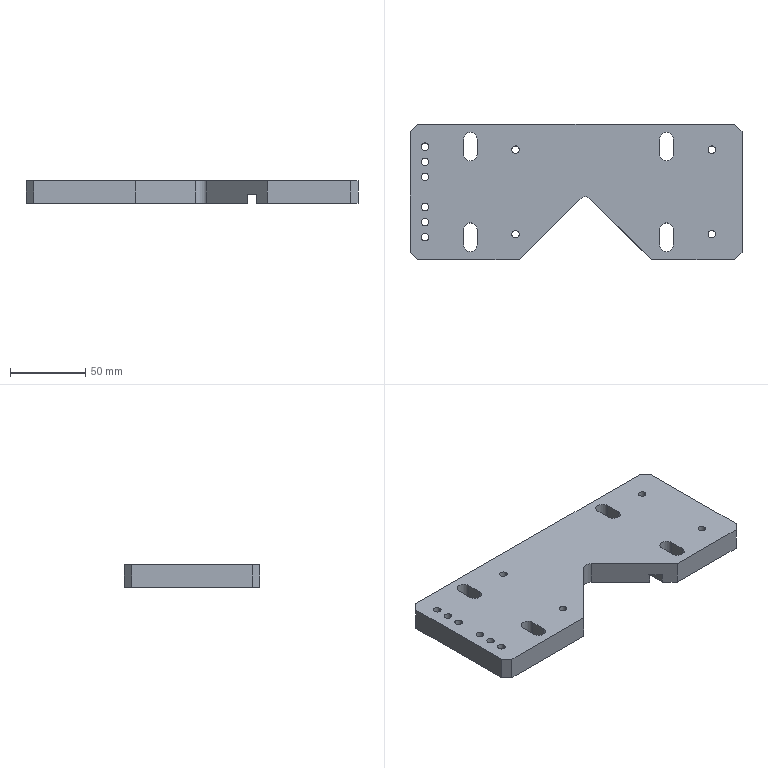Part | SolidWorks | features ICE 3, HoleWzd 2, Chamfer 1, Cut 1, Extrusion 1, Fillet 1 | 1 solid | 58 faces | box 220 x 90 x 15 mm | volume 252154 mm3 | cylinder 31 | plane 25 | cone 2 | commonest cylinder face diameters 5 x22 9 x8 10 x1